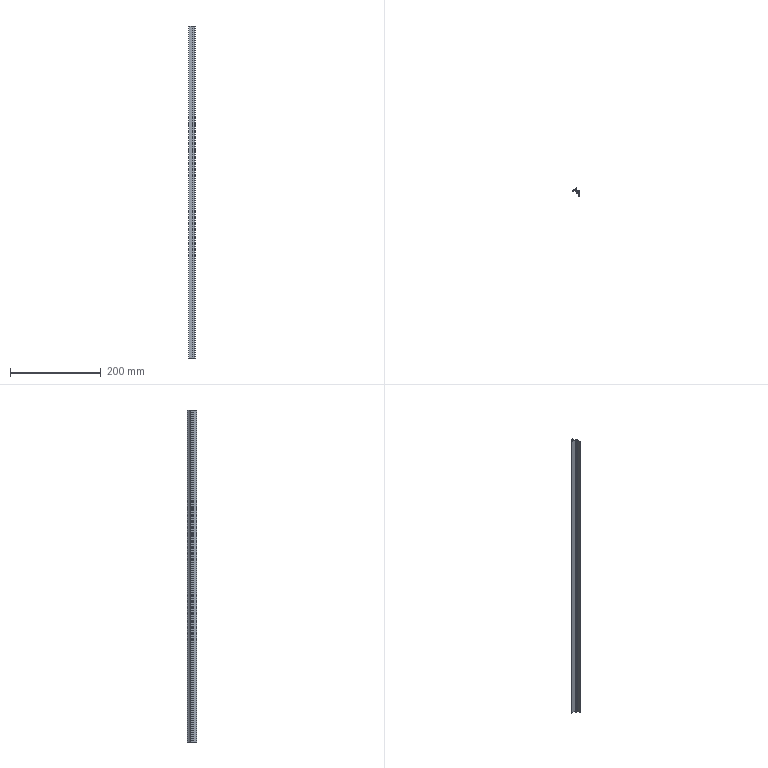Part | SolidWorks | features BaseBody 1, ICE 1, MoveFace 1 | 1 solid | 27 faces | box 14 x 20.3 x 730 mm | volume 37168 mm3 | plane 20 | cylinder 7 | commonest cylinder face diameters 0.387 x2 0.8 x2 0.4 x1 20 x1 22 x1
STEP:
#1=CARTESIAN_POINT('',(-5.304,-0.625,200.));
#2=VERTEX_POINT('',#1);
#3=CARTESIAN_POINT('',(-5.449,-0.8125,200.));
#4=VERTEX_POINT('',#3);
#5=CARTESIAN_POINT('',(-5.255,-0.8125,200.));
#6=DIRECTION('',(0.,0.,1.));
#7=DIRECTION('',(-1.,0.,0.));
#8=AXIS2_PLACEMENT_3D('',#5,#6,#7);
#9=CIRCLE('',#8,0.1937);
#10=EDGE_CURVE('',#2,#4,#9,.T.);
#11=ORIENTED_EDGE('',*,*,#10,.T.);
#12=CARTESIAN_POINT('',(-5.449,-0.8125,-530.));
#13=VERTEX_POINT('',#12);
#14=CARTESIAN_POINT('',(-5.449,-0.8125,230.));
#15=DIRECTION('',(0.,0.,-1.));
#16=VECTOR('',#15,1000.);
#17=LINE('',#14,#16);
#18=EDGE_CURVE('',#4,#13,#17,.T.);
#19=ORIENTED_EDGE('',*,*,#18,.T.);
#20=CARTESIAN_POINT('',(-5.304,-0.625,-530.));
#21=VERTEX_POINT('',#20);
#22=CARTESIAN_POINT('',(-5.255,-0.8125,-530.));
#23=DIRECTION('',(0.,0.,-1.));
#24=DIRECTION('',(1.,0.,0.));
#25=AXIS2_PLACEMENT_3D('',#22,#23,#24);
#26=CIRCLE('',#25,0.1937);
#27=EDGE_CURVE('',#13,#21,#26,.T.);
#28=ORIENTED_EDGE('',*,*,#27,.T.);
#29=CARTESIAN_POINT('',(-5.304,-0.625,230.));
#30=DIRECTION('',(0.,0.,-1.));
#31=VECTOR('',#30,1000.);
#32=LINE('',#29,#31);
#33=EDGE_CURVE('',#2,#21,#32,.T.);
#34=ORIENTED_EDGE('',*,*,#33,.F.);
#35=EDGE_LOOP('',(#11,#19,#28,#34));
#36=FACE_OUTER_BOUND('',#35,.T.);
#37=CARTESIAN_POINT('',(-5.255,-0.8125,230.));
#38=DIRECTION('',(0.,0.,-1.));
#39=DIRECTION('',(-1.,0.,0.));
#40=AXIS2_PLACEMENT_3D('',#37,#38,#39);
#41=CYLINDRICAL_SURFACE('',#40,0.1937);
#42=ADVANCED_FACE('',(#36),#41,.F.);
#43=CARTESIAN_POINT('',(5.,-1.,-530.));
#44=VERTEX_POINT('',#43);
#45=CARTESIAN_POINT('',(5.,-14.3,-530.));
#46=VERTEX_POINT('',#45);
#47=CARTESIAN_POINT('',(5.,29.623,-530.));
#48=DIRECTION('',(0.,-1.,0.));
#49=VECTOR('',#48,1000.);
#50=LINE('',#47,#49);
#51=EDGE_CURVE('',#44,#46,#50,.T.);
#52=ORIENTED_EDGE('',*,*,#51,.F.);
#53=CARTESIAN_POINT('',(5.,-1.,200.));
#54=VERTEX_POINT('',#53);
#55=CARTESIAN_POINT('',(5.,-1.,230.));
#56=DIRECTION('',(0.,0.,-1.));
#57=VECTOR('',#56,1000.);
#58=LINE('',#55,#57);
#59=EDGE_CURVE('',#54,#44,#58,.T.);
#60=ORIENTED_EDGE('',*,*,#59,.F.);
#61=CARTESIAN_POINT('',(5.,-14.3,200.));
#62=VERTEX_POINT('',#61);
#63=CARTESIAN_POINT('',(5.,-14.3,200.));
#64=DIRECTION('',(0.,1.,0.));
#65=VECTOR('',#64,1000.);
#66=LINE('',#63,#65);
#67=EDGE_CURVE('',#62,#54,#66,.T.);
#68=ORIENTED_EDGE('',*,*,#67,.F.);
#69=CARTESIAN_POINT('',(5.,-14.3,230.));
#70=DIRECTION('',(0.,0.,1.));
#71=VECTOR('',#70,1000.);
#72=LINE('',#69,#71);
#73=EDGE_CURVE('',#46,#62,#72,.T.);
#74=ORIENTED_EDGE('',*,*,#73,.F.);
#75=EDGE_LOOP('',(#52,#60,#68,#74));
#76=FACE_OUTER_BOUND('',#75,.T.);
#77=CARTESIAN_POINT('',(5.,-14.3,230.));
#78=DIRECTION('',(-1.,0.,0.));
#79=DIRECTION('',(0.,0.,1.));
#80=AXIS2_PLACEMENT_3D('',#77,#78,#79);
#81=PLANE('',#80);
#82=ADVANCED_FACE('',(#76),#81,.F.);
#83=CARTESIAN_POINT('',(-9.,-2.,-530.));
#84=VERTEX_POINT('',#83);
#85=CARTESIAN_POINT('',(-9.,-2.,200.));
#86=VERTEX_POINT('',#85);
#87=CARTESIAN_POINT('',(-9.,-2.,230.));
#88=DIRECTION('',(0.,0.,1.));
#89=VECTOR('',#88,1000.);
#90=LINE('',#87,#89);
#91=EDGE_CURVE('',#84,#86,#90,.T.);
#92=ORIENTED_EDGE('',*,*,#91,.F.);
#93=CARTESIAN_POINT('',(0.9,-2.,-530.));
#94=VERTEX_POINT('',#93);
#95=CARTESIAN_POINT('',(5.,-2.,-530.));
#96=DIRECTION('',(-1.,0.,0.));
#97=VECTOR('',#96,1000.);
#98=LINE('',#95,#97);
#99=EDGE_CURVE('',#94,#84,#98,.T.);
#100=ORIENTED_EDGE('',*,*,#99,.F.);
#101=CARTESIAN_POINT('',(0.9,-2.,200.));
#102=VERTEX_POINT('',#101);
#103=CARTESIAN_POINT('',(0.9,-2.,230.));
#104=DIRECTION('',(0.,0.,-1.));
#105=VECTOR('',#104,1000.);
#106=LINE('',#103,#105);
#107=EDGE_CURVE('',#102,#94,#106,.T.);
#108=ORIENTED_EDGE('',*,*,#107,.F.);
#109=CARTESIAN_POINT('',(5.,-2.,200.));
#110=DIRECTION('',(1.,0.,0.));
#111=VECTOR('',#110,1000.);
#112=LINE('',#109,#111);
#113=EDGE_CURVE('',#86,#102,#112,.T.);
#114=ORIENTED_EDGE('',*,*,#113,.F.);
#115=EDGE_LOOP('',(#92,#100,#108,#114));
#116=FACE_OUTER_BOUND('',#115,.T.);
#117=CARTESIAN_POINT('',(-9.,-2.,230.));
#118=DIRECTION('',(0.,1.,0.));
#119=DIRECTION('',(0.,0.,1.));
#120=AXIS2_PLACEMENT_3D('',#117,#118,#119);
#121=PLANE('',#120);
#122=ADVANCED_FACE('',(#116),#121,.F.);
#123=CARTESIAN_POINT('',(4.,-6.,200.));
#124=VERTEX_POINT('',#123);
#125=CARTESIAN_POINT('',(4.,-3.,200.));
#126=VERTEX_POINT('',#125);
#127=CARTESIAN_POINT('',(4.,29.623,200.));
#128=DIRECTION('',(0.,1.,0.));
#129=VECTOR('',#128,1000.);
#130=LINE('',#127,#129);
#131=EDGE_CURVE('',#124,#126,#130,.T.);
#132=ORIENTED_EDGE('',*,*,#131,.F.);
#133=CARTESIAN_POINT('',(1.,-6.,200.));
#134=VERTEX_POINT('',#133);
#135=CARTESIAN_POINT('',(5.,-6.,200.));
#136=DIRECTION('',(1.,0.,0.));
#137=VECTOR('',#136,1000.);
#138=LINE('',#135,#137);
#139=EDGE_CURVE('',#134,#124,#138,.T.);
#140=ORIENTED_EDGE('',*,*,#139,.F.);
#141=CARTESIAN_POINT('',(1.,-6.7,200.));
#142=VERTEX_POINT('',#141);
#143=CARTESIAN_POINT('',(1.,-6.,200.));
#144=DIRECTION('',(0.,-1.,0.));
#145=VECTOR('',#144,1000.);
#146=LINE('',#143,#145);
#147=EDGE_CURVE('',#134,#142,#146,.T.);
#148=ORIENTED_EDGE('',*,*,#147,.T.);
#149=CARTESIAN_POINT('',(-1.7,-6.7,200.));
#150=VERTEX_POINT('',#149);
#151=CARTESIAN_POINT('',(5.,-6.7,200.));
#152=DIRECTION('',(1.,0.,0.));
#153=VECTOR('',#152,1000.);
#154=LINE('',#151,#153);
#155=EDGE_CURVE('',#150,#142,#154,.T.);
#156=ORIENTED_EDGE('',*,*,#155,.F.);
#157=CARTESIAN_POINT('',(-1.7,-7.7,200.));
#158=VERTEX_POINT('',#157);
#159=CARTESIAN_POINT('',(-1.7,-6.7,200.));
#160=DIRECTION('',(0.,-1.,0.));
#161=VECTOR('',#160,1000.);
#162=LINE('',#159,#161);
#163=EDGE_CURVE('',#150,#158,#162,.T.);
#164=ORIENTED_EDGE('',*,*,#163,.T.);
#165=CARTESIAN_POINT('',(4.,-7.7,200.));
#166=VERTEX_POINT('',#165);
#167=CARTESIAN_POINT('',(5.,-7.7,200.));
#168=DIRECTION('',(-1.,0.,0.));
#169=VECTOR('',#168,1000.);
#170=LINE('',#167,#169);
#171=EDGE_CURVE('',#166,#158,#170,.T.);
#172=ORIENTED_EDGE('',*,*,#171,.F.);
#173=CARTESIAN_POINT('',(4.,-14.3,200.));
#174=VERTEX_POINT('',#173);
#175=CARTESIAN_POINT('',(4.,29.623,200.));
#176=DIRECTION('',(0.,1.,0.));
#177=VECTOR('',#176,1000.);
#178=LINE('',#175,#177);
#179=EDGE_CURVE('',#174,#166,#178,.T.);
#180=ORIENTED_EDGE('',*,*,#179,.F.);
#181=CARTESIAN_POINT('',(5.,-14.3,200.));
#182=DIRECTION('',(-1.,0.,0.));
#183=VECTOR('',#182,1000.);
#184=LINE('',#181,#183);
#185=EDGE_CURVE('',#62,#174,#184,.T.);
#186=ORIENTED_EDGE('',*,*,#185,.F.);
#187=ORIENTED_EDGE('',*,*,#67,.T.);
#188=CARTESIAN_POINT('',(-5.207,-1.,200.));
#189=VERTEX_POINT('',#188);
#190=CARTESIAN_POINT('',(5.,-1.,200.));
#191=DIRECTION('',(1.,0.,0.));
#192=VECTOR('',#191,1000.);
#193=LINE('',#190,#192);
#194=EDGE_CURVE('',#189,#54,#193,.T.);
#195=ORIENTED_EDGE('',*,*,#194,.F.);
#196=CARTESIAN_POINT('',(-5.255,-0.8125,200.));
#197=DIRECTION('',(0.,0.,1.));
#198=DIRECTION('',(-1.,0.,0.));
#199=AXIS2_PLACEMENT_3D('',#196,#197,#198);
#200=CIRCLE('',#199,0.1937);
#201=EDGE_CURVE('',#4,#189,#200,.T.);
#202=ORIENTED_EDGE('',*,*,#201,.F.);
#203=ORIENTED_EDGE('',*,*,#10,.F.);
#204=CARTESIAN_POINT('',(-1.368,3.063,200.));
#205=VERTEX_POINT('',#204);
#206=CARTESIAN_POINT('',(-10.628,9.,200.));
#207=DIRECTION('',(0.,0.,1.));
#208=DIRECTION('',(-1.,0.,0.));
#209=AXIS2_PLACEMENT_3D('',#206,#207,#208);
#210=CIRCLE('',#209,11.);
#211=EDGE_CURVE('',#2,#205,#210,.T.);
#212=ORIENTED_EDGE('',*,*,#211,.T.);
#213=CARTESIAN_POINT('',(-1.,2.955,200.));
#214=VERTEX_POINT('',#213);
#215=CARTESIAN_POINT('',(-1.2,2.955,200.));
#216=DIRECTION('',(0.,0.,1.));
#217=DIRECTION('',(-1.,0.,0.));
#218=AXIS2_PLACEMENT_3D('',#215,#216,#217);
#219=CIRCLE('',#218,0.2);
#220=EDGE_CURVE('',#214,#205,#219,.T.);
#221=ORIENTED_EDGE('',*,*,#220,.F.);
#222=CARTESIAN_POINT('',(-1.,1.5,200.));
#223=VERTEX_POINT('',#222);
#224=CARTESIAN_POINT('',(-1.,2.955,200.));
#225=DIRECTION('',(0.,1.,0.));
#226=VECTOR('',#225,1000.);
#227=LINE('',#224,#226);
#228=EDGE_CURVE('',#223,#214,#227,.T.);
#229=ORIENTED_EDGE('',*,*,#228,.F.);
#230=CARTESIAN_POINT('',(0.,1.5,200.));
#231=VERTEX_POINT('',#230);
#232=CARTESIAN_POINT('',(-1.,1.5,200.));
#233=DIRECTION('',(-1.,0.,0.));
#234=VECTOR('',#233,1000.);
#235=LINE('',#232,#234);
#236=EDGE_CURVE('',#231,#223,#235,.T.);
#237=ORIENTED_EDGE('',*,*,#236,.F.);
#238=CARTESIAN_POINT('',(0.,6.,200.));
#239=VERTEX_POINT('',#238);
#240=CARTESIAN_POINT('',(0.,1.5,200.));
#241=DIRECTION('',(0.,-1.,0.));
#242=VECTOR('',#241,1000.);
#243=LINE('',#240,#242);
#244=EDGE_CURVE('',#239,#231,#243,.T.);
#245=ORIENTED_EDGE('',*,*,#244,.F.);
#246=CARTESIAN_POINT('',(-0.8,6.,200.));
#247=VERTEX_POINT('',#246);
#248=CARTESIAN_POINT('',(0.,6.,200.));
#249=DIRECTION('',(1.,0.,0.));
#250=VECTOR('',#249,1000.);
#251=LINE('',#248,#250);
#252=EDGE_CURVE('',#247,#239,#251,.T.);
#253=ORIENTED_EDGE('',*,*,#252,.F.);
#254=CARTESIAN_POINT('',(-1.178,5.731,200.));
#255=VERTEX_POINT('',#254);
#256=CARTESIAN_POINT('',(-0.8,5.6,200.));
#257=DIRECTION('',(0.,0.,1.));
#258=DIRECTION('',(-1.,0.,0.));
#259=AXIS2_PLACEMENT_3D('',#256,#257,#258);
#260=CIRCLE('',#259,0.4);
#261=EDGE_CURVE('',#247,#255,#260,.T.);
#262=ORIENTED_EDGE('',*,*,#261,.T.);
#263=CARTESIAN_POINT('',(-8.678,-0.8077,200.));
#264=VERTEX_POINT('',#263);
#265=CARTESIAN_POINT('',(-10.628,9.,200.));
#266=DIRECTION('',(0.,0.,1.));
#267=DIRECTION('',(-1.,0.,0.));
#268=AXIS2_PLACEMENT_3D('',#265,#266,#267);
#269=CIRCLE('',#268,10.);
#270=EDGE_CURVE('',#264,#255,#269,.T.);
#271=ORIENTED_EDGE('',*,*,#270,.F.);
#272=CARTESIAN_POINT('',(-9.,-1.2,200.));
#273=VERTEX_POINT('',#272);
#274=CARTESIAN_POINT('',(-8.6,-1.2,200.));
#275=DIRECTION('',(0.,0.,1.));
#276=DIRECTION('',(-1.,0.,0.));
#277=AXIS2_PLACEMENT_3D('',#274,#275,#276);
#278=CIRCLE('',#277,0.4);
#279=EDGE_CURVE('',#264,#273,#278,.T.);
#280=ORIENTED_EDGE('',*,*,#279,.T.);
#281=CARTESIAN_POINT('',(-9.,8.,200.));
#282=DIRECTION('',(0.,-1.,0.));
#283=VECTOR('',#282,1000.);
#284=LINE('',#281,#283);
#285=EDGE_CURVE('',#273,#86,#284,.T.);
#286=ORIENTED_EDGE('',*,*,#285,.T.);
#287=ORIENTED_EDGE('',*,*,#113,.T.);
#288=CARTESIAN_POINT('',(0.9,-3.,200.));
#289=VERTEX_POINT('',#288);
#290=CARTESIAN_POINT('',(0.9,29.623,200.));
#291=DIRECTION('',(0.,1.,0.));
#292=VECTOR('',#291,1000.);
#293=LINE('',#290,#292);
#294=EDGE_CURVE('',#289,#102,#293,.T.);
#295=ORIENTED_EDGE('',*,*,#294,.F.);
#296=CARTESIAN_POINT('',(5.,-3.,200.));
#297=DIRECTION('',(-1.,0.,0.));
#298=VECTOR('',#297,1000.);
#299=LINE('',#296,#298);
#300=EDGE_CURVE('',#126,#289,#299,.T.);
#301=ORIENTED_EDGE('',*,*,#300,.F.);
#302=EDGE_LOOP('',(#132,#140,#148,#156,#164,#172,#180,#186,#187,#195,#202,#203,#212,#221,#229,#237,#245,#253,#262,#271,#280,#286,#287,#295,#301));
#303=FACE_OUTER_BOUND('',#302,.T.);
#304=CARTESIAN_POINT('',(5.,29.623,200.));
#305=DIRECTION('',(0.,0.,-1.));
#306=DIRECTION('',(-1.,0.,0.));
#307=AXIS2_PLACEMENT_3D('',#304,#305,#306);
#308=PLANE('',#307);
#309=ADVANCED_FACE('',(#303),#308,.F.);
#310=ORIENTED_EDGE('',*,*,#185,.T.);
#311=CARTESIAN_POINT('',(4.,-14.3,-530.));
#312=VERTEX_POINT('',#311);
#313=CARTESIAN_POINT('',(4.,-14.3,230.));
#314=DIRECTION('',(0.,0.,1.));
#315=VECTOR('',#314,1000.);
#316=LINE('',#313,#315);
#317=EDGE_CURVE('',#312,#174,#316,.T.);
#318=ORIENTED_EDGE('',*,*,#317,.F.);
#319=CARTESIAN_POINT('',(5.,-14.3,-530.));
#320=DIRECTION('',(-1.,0.,0.));
#321=VECTOR('',#320,1000.);
#322=LINE('',#319,#321);
#323=EDGE_CURVE('',#46,#312,#322,.T.);
#324=ORIENTED_EDGE('',*,*,#323,.F.);
#325=ORIENTED_EDGE('',*,*,#73,.T.);
#326=EDGE_LOOP('',(#310,#318,#324,#325));
#327=FACE_OUTER_BOUND('',#326,.T.);
#328=CARTESIAN_POINT('',(4.,-14.3,230.));
#329=DIRECTION('',(0.,1.,0.));
#330=DIRECTION('',(0.,0.,1.));
#331=AXIS2_PLACEMENT_3D('',#328,#329,#330);
#332=PLANE('',#331);
#333=ADVANCED_FACE('',(#327),#332,.F.);
#334=ORIENTED_EDGE('',*,*,#51,.T.);
#335=ORIENTED_EDGE('',*,*,#323,.T.);
#336=CARTESIAN_POINT('',(4.,-7.7,-530.));
#337=VERTEX_POINT('',#336);
#338=CARTESIAN_POINT('',(4.,-7.7,-530.));
#339=DIRECTION('',(0.,-1.,0.));
#340=VECTOR('',#339,1000.);
#341=LINE('',#338,#340);
#342=EDGE_CURVE('',#337,#312,#341,.T.);
#343=ORIENTED_EDGE('',*,*,#342,.F.);
#344=CARTESIAN_POINT('',(-1.7,-7.7,-530.));
#345=VERTEX_POINT('',#344);
#346=CARTESIAN_POINT('',(-1.7,-7.7,-530.));
#347=DIRECTION('',(1.,0.,0.));
#348=VECTOR('',#347,1000.);
#349=LINE('',#346,#348);
#350=EDGE_CURVE('',#345,#337,#349,.T.);
#351=ORIENTED_EDGE('',*,*,#350,.F.);
#352=CARTESIAN_POINT('',(-1.7,-6.7,-530.));
#353=VERTEX_POINT('',#352);
#354=CARTESIAN_POINT('',(-1.7,29.623,-530.));
#355=DIRECTION('',(0.,1.,0.));
#356=VECTOR('',#355,1000.);
#357=LINE('',#354,#356);
#358=EDGE_CURVE('',#345,#353,#357,.T.);
#359=ORIENTED_EDGE('',*,*,#358,.T.);
#360=CARTESIAN_POINT('',(1.,-6.7,-530.));
#361=VERTEX_POINT('',#360);
#362=CARTESIAN_POINT('',(1.,-6.7,-530.));
#363=DIRECTION('',(-1.,0.,0.));
#364=VECTOR('',#363,1000.);
#365=LINE('',#362,#364);
#366=EDGE_CURVE('',#361,#353,#365,.T.);
#367=ORIENTED_EDGE('',*,*,#366,.F.);
#368=CARTESIAN_POINT('',(1.,-6.,-530.));
#369=VERTEX_POINT('',#368);
#370=CARTESIAN_POINT('',(1.,29.623,-530.));
#371=DIRECTION('',(0.,1.,0.));
#372=VECTOR('',#371,1000.);
#373=LINE('',#370,#372);
#374=EDGE_CURVE('',#361,#369,#373,.T.);
#375=ORIENTED_EDGE('',*,*,#374,.T.);
#376=CARTESIAN_POINT('',(4.,-6.,-530.));
#377=VERTEX_POINT('',#376);
#378=CARTESIAN_POINT('',(4.,-6.,-530.));
#379=DIRECTION('',(-1.,0.,0.));
#380=VECTOR('',#379,1000.);
#381=LINE('',#378,#380);
#382=EDGE_CURVE('',#377,#369,#381,.T.);
#383=ORIENTED_EDGE('',*,*,#382,.F.);
#384=CARTESIAN_POINT('',(4.,-3.,-530.));
#385=VERTEX_POINT('',#384);
#386=CARTESIAN_POINT('',(4.,-3.,-530.));
#387=DIRECTION('',(0.,-1.,0.));
#388=VECTOR('',#387,1000.);
#389=LINE('',#386,#388);
#390=EDGE_CURVE('',#385,#377,#389,.T.);
#391=ORIENTED_EDGE('',*,*,#390,.F.);
#392=CARTESIAN_POINT('',(0.9,-3.,-530.));
#393=VERTEX_POINT('',#392);
#394=CARTESIAN_POINT('',(0.9,-3.,-530.));
#395=DIRECTION('',(1.,0.,0.));
#396=VECTOR('',#395,1000.);
#397=LINE('',#394,#396);
#398=EDGE_CURVE('',#393,#385,#397,.T.);
#399=ORIENTED_EDGE('',*,*,#398,.F.);
#400=CARTESIAN_POINT('',(0.9,-2.,-530.));
#401=DIRECTION('',(0.,-1.,0.));
#402=VECTOR('',#401,1000.);
#403=LINE('',#400,#402);
#404=EDGE_CURVE('',#94,#393,#403,.T.);
#405=ORIENTED_EDGE('',*,*,#404,.F.);
#406=ORIENTED_EDGE('',*,*,#99,.T.);
#407=CARTESIAN_POINT('',(-9.,-1.2,-530.));
#408=VERTEX_POINT('',#407);
#409=CARTESIAN_POINT('',(-9.,-1.2,-530.));
#410=DIRECTION('',(0.,-1.,0.));
#411=VECTOR('',#410,1000.);
#412=LINE('',#409,#411);
#413=EDGE_CURVE('',#408,#84,#412,.T.);
#414=ORIENTED_EDGE('',*,*,#413,.F.);
#415=CARTESIAN_POINT('',(-8.678,-0.8077,-530.));
#416=VERTEX_POINT('',#415);
#417=CARTESIAN_POINT('',(-8.6,-1.2,-530.));
#418=DIRECTION('',(0.,0.,-1.));
#419=DIRECTION('',(1.,0.,0.));
#420=AXIS2_PLACEMENT_3D('',#417,#418,#419);
#421=CIRCLE('',#420,0.4);
#422=EDGE_CURVE('',#408,#416,#421,.T.);
#423=ORIENTED_EDGE('',*,*,#422,.T.);
#424=CARTESIAN_POINT('',(-1.178,5.731,-530.));
#425=VERTEX_POINT('',#424);
#426=CARTESIAN_POINT('',(-10.628,9.,-530.));
#427=DIRECTION('',(0.,0.,-1.));
#428=DIRECTION('',(1.,0.,0.));
#429=AXIS2_PLACEMENT_3D('',#426,#427,#428);
#430=CIRCLE('',#429,10.);
#431=EDGE_CURVE('',#425,#416,#430,.T.);
#432=ORIENTED_EDGE('',*,*,#431,.F.);
#433=CARTESIAN_POINT('',(-0.8,6.,-530.));
#434=VERTEX_POINT('',#433);
#435=CARTESIAN_POINT('',(-0.8,5.6,-530.));
#436=DIRECTION('',(0.,0.,-1.));
#437=DIRECTION('',(1.,0.,0.));
#438=AXIS2_PLACEMENT_3D('',#435,#436,#437);
#439=CIRCLE('',#438,0.4);
#440=EDGE_CURVE('',#425,#434,#439,.T.);
#441=ORIENTED_EDGE('',*,*,#440,.T.);
#442=CARTESIAN_POINT('',(0.,6.,-530.));
#443=VERTEX_POINT('',#442);
#444=CARTESIAN_POINT('',(0.,6.,-530.));
#445=DIRECTION('',(-1.,0.,0.));
#446=VECTOR('',#445,1000.);
#447=LINE('',#444,#446);
#448=EDGE_CURVE('',#443,#434,#447,.T.);
#449=ORIENTED_EDGE('',*,*,#448,.F.);
#450=CARTESIAN_POINT('',(0.,1.5,-530.));
#451=VERTEX_POINT('',#450);
#452=CARTESIAN_POINT('',(0.,1.5,-530.));
#453=DIRECTION('',(0.,1.,0.));
#454=VECTOR('',#453,1000.);
#455=LINE('',#452,#454);
#456=EDGE_CURVE('',#451,#443,#455,.T.);
#457=ORIENTED_EDGE('',*,*,#456,.F.);
#458=CARTESIAN_POINT('',(-1.,1.5,-530.));
#459=VERTEX_POINT('',#458);
#460=CARTESIAN_POINT('',(-1.,1.5,-530.));
#461=DIRECTION('',(1.,0.,0.));
#462=VECTOR('',#461,1000.);
#463=LINE('',#460,#462);
#464=EDGE_CURVE('',#459,#451,#463,.T.);
#465=ORIENTED_EDGE('',*,*,#464,.F.);
#466=CARTESIAN_POINT('',(-1.,2.955,-530.));
#467=VERTEX_POINT('',#466);
#468=CARTESIAN_POINT('',(-1.,2.955,-530.));
#469=DIRECTION('',(0.,-1.,0.));
#470=VECTOR('',#469,1000.);
#471=LINE('',#468,#470);
#472=EDGE_CURVE('',#467,#459,#471,.T.);
#473=ORIENTED_EDGE('',*,*,#472,.F.);
#474=CARTESIAN_POINT('',(-1.368,3.063,-530.));
#475=VERTEX_POINT('',#474);
#476=CARTESIAN_POINT('',(-1.2,2.955,-530.));
#477=DIRECTION('',(0.,0.,-1.));
#478=DIRECTION('',(1.,0.,0.));
#479=AXIS2_PLACEMENT_3D('',#476,#477,#478);
#480=CIRCLE('',#479,0.2);
#481=EDGE_CURVE('',#475,#467,#480,.T.);
#482=ORIENTED_EDGE('',*,*,#481,.F.);
#483=CARTESIAN_POINT('',(-10.628,9.,-530.));
#484=DIRECTION('',(0.,0.,-1.));
#485=DIRECTION('',(1.,0.,0.));
#486=AXIS2_PLACEMENT_3D('',#483,#484,#485);
#487=CIRCLE('',#486,11.);
#488=EDGE_CURVE('',#475,#21,#487,.T.);
#489=ORIENTED_EDGE('',*,*,#488,.T.);
#490=ORIENTED_EDGE('',*,*,#27,.F.);
#491=CARTESIAN_POINT('',(-5.207,-1.,-530.));
#492=VERTEX_POINT('',#491);
#493=CARTESIAN_POINT('',(-5.255,-0.8125,-530.));
#494=DIRECTION('',(0.,0.,-1.));
#495=DIRECTION('',(1.,0.,0.));
#496=AXIS2_PLACEMENT_3D('',#493,#494,#495);
#497=CIRCLE('',#496,0.1937);
#498=EDGE_CURVE('',#492,#13,#497,.T.);
#499=ORIENTED_EDGE('',*,*,#498,.F.);
#500=CARTESIAN_POINT('',(5.,-1.,-530.));
#501=DIRECTION('',(-1.,0.,0.));
#502=VECTOR('',#501,1000.);
#503=LINE('',#500,#502);
#504=EDGE_CURVE('',#44,#492,#503,.T.);
#505=ORIENTED_EDGE('',*,*,#504,.F.);
#506=EDGE_LOOP('',(#334,#335,#343,#351,#359,#367,#375,#383,#391,#399,#405,#406,#414,#423,#432,#441,#449,#457,#465,#473,#482,#489,#490,#499,#505));
#507=FACE_OUTER_BOUND('',#506,.T.);
#508=CARTESIAN_POINT('',(5.,29.623,-530.));
#509=DIRECTION('',(0.,0.,1.));
#510=DIRECTION('',(1.,0.,0.));
#511=AXIS2_PLACEMENT_3D('',#508,#509,#510);
#512=PLANE('',#511);
#513=ADVANCED_FACE('',(#507),#512,.F.);
#514=ORIENTED_EDGE('',*,*,#59,.T.);
#515=ORIENTED_EDGE('',*,*,#504,.T.);
#516=CARTESIAN_POINT('',(-5.207,-1.,230.));
#517=DIRECTION('',(0.,0.,-1.));
#518=VECTOR('',#517,1000.);
#519=LINE('',#516,#518);
#520=EDGE_CURVE('',#189,#492,#519,.T.);
#521=ORIENTED_EDGE('',*,*,#520,.F.);
#522=ORIENTED_EDGE('',*,*,#194,.T.);
#523=EDGE_LOOP('',(#514,#515,#521,#522));
#524=FACE_OUTER_BOUND('',#523,.T.);
#525=CARTESIAN_POINT('',(5.,-1.,230.));
#526=DIRECTION('',(0.,-1.,0.));
#527=DIRECTION('',(0.,0.,-1.));
#528=AXIS2_PLACEMENT_3D('',#525,#526,#527);
#529=PLANE('',#528);
#530=ADVANCED_FACE('',(#524),#529,.F.);
#531=CARTESIAN_POINT('',(-9.,-1.2,230.));
#532=DIRECTION('',(0.,0.,1.));
#533=VECTOR('',#532,1000.);
#534=LINE('',#531,#533);
#535=EDGE_CURVE('',#408,#273,#534,.T.);
#536=ORIENTED_EDGE('',*,*,#535,.F.);
#537=ORIENTED_EDGE('',*,*,#413,.T.);
#538=ORIENTED_EDGE('',*,*,#91,.T.);
#539=ORIENTED_EDGE('',*,*,#285,.F.);
#540=EDGE_LOOP('',(#536,#537,#538,#539));
#541=FACE_OUTER_BOUND('',#540,.T.);
#542=CARTESIAN_POINT('',(-9.,-1.2,230.));
#543=DIRECTION('',(1.,0.,0.));
#544=DIRECTION('',(0.,0.,-1.));
#545=AXIS2_PLACEMENT_3D('',#542,#543,#544);
#546=PLANE('',#545);
#547=ADVANCED_FACE('',(#541),#546,.F.);
#548=ORIENTED_EDGE('',*,*,#294,.T.);
#549=ORIENTED_EDGE('',*,*,#107,.T.);
#550=ORIENTED_EDGE('',*,*,#404,.T.);
#551=CARTESIAN_POINT('',(0.9,-3.,230.));
#552=DIRECTION('',(0.,0.,-1.));
#553=VECTOR('',#552,1000.);
#554=LINE('',#551,#553);
#555=EDGE_CURVE('',#289,#393,#554,.T.);
#556=ORIENTED_EDGE('',*,*,#555,.F.);
#557=EDGE_LOOP('',(#548,#549,#550,#556));
#558=FACE_OUTER_BOUND('',#557,.T.);
#559=CARTESIAN_POINT('',(0.9,-2.,230.));
#560=DIRECTION('',(1.,0.,0.));
#561=DIRECTION('',(0.,0.,-1.));
#562=AXIS2_PLACEMENT_3D('',#559,#560,#561);
#563=PLANE('',#562);
#564=ADVANCED_FACE('',(#558),#563,.F.);
#565=ORIENTED_EDGE('',*,*,#300,.T.);
#566=ORIENTED_EDGE('',*,*,#555,.T.);
#567=ORIENTED_EDGE('',*,*,#398,.T.);
#568=CARTESIAN_POINT('',(4.,-3.,230.));
#569=DIRECTION('',(0.,0.,-1.));
#570=VECTOR('',#569,1000.);
#571=LINE('',#568,#570);
#572=EDGE_CURVE('',#126,#385,#571,.T.);
#573=ORIENTED_EDGE('',*,*,#572,.F.);
#574=EDGE_LOOP('',(#565,#566,#567,#573));
#575=FACE_OUTER_BOUND('',#574,.T.);
#576=CARTESIAN_POINT('',(0.9,-3.,230.));
#577=DIRECTION('',(0.,1.,0.));
#578=DIRECTION('',(0.,0.,1.));
#579=AXIS2_PLACEMENT_3D('',#576,#577,#578);
#580=PLANE('',#579);
#581=ADVANCED_FACE('',(#575),#580,.F.);
#582=ORIENTED_EDGE('',*,*,#131,.T.);
#583=ORIENTED_EDGE('',*,*,#572,.T.);
#584=ORIENTED_EDGE('',*,*,#390,.T.);
#585=CARTESIAN_POINT('',(4.,-6.,230.));
#586=DIRECTION('',(0.,0.,-1.));
#587=VECTOR('',#586,1000.);
#588=LINE('',#585,#587);
#589=EDGE_CURVE('',#124,#377,#588,.T.);
#590=ORIENTED_EDGE('',*,*,#589,.F.);
#591=EDGE_LOOP('',(#582,#583,#584,#590));
#592=FACE_OUTER_BOUND('',#591,.T.);
#593=CARTESIAN_POINT('',(4.,-3.,230.));
#594=DIRECTION('',(1.,0.,0.));
#595=DIRECTION('',(0.,0.,-1.));
#596=AXIS2_PLACEMENT_3D('',#593,#594,#595);
#597=PLANE('',#596);
#598=ADVANCED_FACE('',(#592),#597,.F.);
#599=ORIENTED_EDGE('',*,*,#139,.T.);
#600=ORIENTED_EDGE('',*,*,#589,.T.);
#601=ORIENTED_EDGE('',*,*,#382,.T.);
#602=CARTESIAN_POINT('',(1.,-6.,230.));
#603=DIRECTION('',(0.,0.,-1.));
#604=VECTOR('',#603,1000.);
#605=LINE('',#602,#604);
#606=EDGE_CURVE('',#134,#369,#605,.T.);
#607=ORIENTED_EDGE('',*,*,#606,.F.);
#608=EDGE_LOOP('',(#599,#600,#601,#607));
#609=FACE_OUTER_BOUND('',#608,.T.);
#610=CARTESIAN_POINT('',(4.,-6.,230.));
#611=DIRECTION('',(0.,-1.,0.));
#612=DIRECTION('',(0.,0.,-1.));
#613=AXIS2_PLACEMENT_3D('',#610,#611,#612);
#614=PLANE('',#613);
#615=ADVANCED_FACE('',(#609),#614,.F.);
#616=ORIENTED_EDGE('',*,*,#155,.T.);
#617=CARTESIAN_POINT('',(1.,-6.7,230.));
#618=DIRECTION('',(0.,0.,1.));
#619=VECTOR('',#618,1000.);
#620=LINE('',#617,#619);
#621=EDGE_CURVE('',#361,#142,#620,.T.);
#622=ORIENTED_EDGE('',*,*,#621,.F.);
#623=ORIENTED_EDGE('',*,*,#366,.T.);
#624=CARTESIAN_POINT('',(-1.7,-6.7,230.));
#625=DIRECTION('',(0.,0.,-1.));
#626=VECTOR('',#625,1000.);
#627=LINE('',#624,#626);
#628=EDGE_CURVE('',#150,#353,#627,.T.);
#629=ORIENTED_EDGE('',*,*,#628,.F.);
#630=EDGE_LOOP('',(#616,#622,#623,#629));
#631=FACE_OUTER_BOUND('',#630,.T.);
#632=CARTESIAN_POINT('',(1.,-6.7,230.));
#633=DIRECTION('',(0.,-1.,0.));
#634=DIRECTION('',(0.,0.,-1.));
#635=AXIS2_PLACEMENT_3D('',#632,#633,#634);
#636=PLANE('',#635);
#637=ADVANCED_FACE('',(#631),#636,.F.);
#638=ORIENTED_EDGE('',*,*,#171,.T.);
#639=CARTESIAN_POINT('',(-1.7,-7.7,230.));
#640=DIRECTION('',(0.,0.,1.));
#641=VECTOR('',#640,1000.);
#642=LINE('',#639,#641);
#643=EDGE_CURVE('',#345,#158,#642,.T.);
#644=ORIENTED_EDGE('',*,*,#643,.F.);
#645=ORIENTED_EDGE('',*,*,#350,.T.);
#646=CARTESIAN_POINT('',(4.,-7.7,230.));
#647=DIRECTION('',(0.,0.,-1.));
#648=VECTOR('',#647,1000.);
#649=LINE('',#646,#648);
#650=EDGE_CURVE('',#166,#337,#649,.T.);
#651=ORIENTED_EDGE('',*,*,#650,.F.);
#652=EDGE_LOOP('',(#638,#644,#645,#651));
#653=FACE_OUTER_BOUND('',#652,.T.);
#654=CARTESIAN_POINT('',(-1.7,-7.7,230.));
#655=DIRECTION('',(0.,1.,0.));
#656=DIRECTION('',(0.,0.,1.));
#657=AXIS2_PLACEMENT_3D('',#654,#655,#656);
#658=PLANE('',#657);
#659=ADVANCED_FACE('',(#653),#658,.F.);
#660=ORIENTED_EDGE('',*,*,#179,.T.);
#661=ORIENTED_EDGE('',*,*,#650,.T.);
#662=ORIENTED_EDGE('',*,*,#342,.T.);
#663=ORIENTED_EDGE('',*,*,#317,.T.);
#664=EDGE_LOOP('',(#660,#661,#662,#663));
#665=FACE_OUTER_BOUND('',#664,.T.);
#666=CARTESIAN_POINT('',(4.,-7.7,230.));
#667=DIRECTION('',(1.,0.,0.));
#668=DIRECTION('',(0.,0.,-1.));
#669=AXIS2_PLACEMENT_3D('',#666,#667,#668);
#670=PLANE('',#669);
#671=ADVANCED_FACE('',(#665),#670,.F.);
#672=ORIENTED_EDGE('',*,*,#18,.F.);
#673=ORIENTED_EDGE('',*,*,#201,.T.);
#674=ORIENTED_EDGE('',*,*,#520,.T.);
#675=ORIENTED_EDGE('',*,*,#498,.T.);
#676=EDGE_LOOP('',(#672,#673,#674,#675));
#677=FACE_OUTER_BOUND('',#676,.T.);
#678=CARTESIAN_POINT('',(-5.255,-0.8125,230.));
#679=DIRECTION('',(0.,0.,-1.));
#680=DIRECTION('',(-1.,0.,0.));
#681=AXIS2_PLACEMENT_3D('',#678,#679,#680);
#682=CYLINDRICAL_SURFACE('',#681,0.1937);
#683=ADVANCED_FACE('',(#677),#682,.F.);
#684=CARTESIAN_POINT('',(-1.,2.955,230.));
#685=DIRECTION('',(0.,0.,1.));
#686=VECTOR('',#685,1000.);
#687=LINE('',#684,#686);
#688=EDGE_CURVE('',#467,#214,#687,.T.);
#689=ORIENTED_EDGE('',*,*,#688,.F.);
#690=ORIENTED_EDGE('',*,*,#472,.T.);
#691=CARTESIAN_POINT('',(-1.,1.5,230.));
#692=DIRECTION('',(0.,0.,-1.));
#693=VECTOR('',#692,1000.);
#694=LINE('',#691,#693);
#695=EDGE_CURVE('',#223,#459,#694,.T.);
#696=ORIENTED_EDGE('',*,*,#695,.F.);
#697=ORIENTED_EDGE('',*,*,#228,.T.);
#698=EDGE_LOOP('',(#689,#690,#696,#697));
#699=FACE_OUTER_BOUND('',#698,.T.);
#700=CARTESIAN_POINT('',(-1.,2.955,230.));
#701=DIRECTION('',(1.,0.,0.));
#702=DIRECTION('',(0.,0.,-1.));
#703=AXIS2_PLACEMENT_3D('',#700,#701,#702);
#704=PLANE('',#703);
#705=ADVANCED_FACE('',(#699),#704,.F.);
#706=ORIENTED_EDGE('',*,*,#488,.F.);
#707=CARTESIAN_POINT('',(-1.368,3.063,230.));
#708=DIRECTION('',(0.,0.,1.));
#709=VECTOR('',#708,1000.);
#710=LINE('',#707,#709);
#711=EDGE_CURVE('',#475,#205,#710,.T.);
#712=ORIENTED_EDGE('',*,*,#711,.T.);
#713=ORIENTED_EDGE('',*,*,#211,.F.);
#714=ORIENTED_EDGE('',*,*,#33,.T.);
#715=EDGE_LOOP('',(#706,#712,#713,#714));
#716=FACE_OUTER_BOUND('',#715,.T.);
#717=CARTESIAN_POINT('',(-10.628,9.,230.));
#718=DIRECTION('',(0.,0.,-1.));
#719=DIRECTION('',(-1.,0.,0.));
#720=AXIS2_PLACEMENT_3D('',#717,#718,#719);
#721=CYLINDRICAL_SURFACE('',#720,11.);
#722=ADVANCED_FACE('',(#716),#721,.T.);
#723=CARTESIAN_POINT('',(-1.178,5.731,230.));
#724=DIRECTION('',(0.,0.,1.));
#725=VECTOR('',#724,1000.);
#726=LINE('',#723,#725);
#727=EDGE_CURVE('',#425,#255,#726,.T.);
#728=ORIENTED_EDGE('',*,*,#727,.F.);
#729=ORIENTED_EDGE('',*,*,#431,.T.);
#730=CARTESIAN_POINT('',(-8.678,-0.8077,230.));
#731=DIRECTION('',(0.,0.,-1.));
#732=VECTOR('',#731,1000.);
#733=LINE('',#730,#732);
#734=EDGE_CURVE('',#264,#416,#733,.T.);
#735=ORIENTED_EDGE('',*,*,#734,.F.);
#736=ORIENTED_EDGE('',*,*,#270,.T.);
#737=EDGE_LOOP('',(#728,#729,#735,#736));
#738=FACE_OUTER_BOUND('',#737,.T.);
#739=CARTESIAN_POINT('',(-10.628,9.,230.));
#740=DIRECTION('',(0.,0.,-1.));
#741=DIRECTION('',(-1.,0.,0.));
#742=AXIS2_PLACEMENT_3D('',#739,#740,#741);
#743=CYLINDRICAL_SURFACE('',#742,10.);
#744=ADVANCED_FACE('',(#738),#743,.F.);
#745=CARTESIAN_POINT('',(0.,1.5,230.));
#746=DIRECTION('',(0.,0.,1.));
#747=VECTOR('',#746,1000.);
#748=LINE('',#745,#747);
#749=EDGE_CURVE('',#451,#231,#748,.T.);
#750=ORIENTED_EDGE('',*,*,#749,.F.);
#751=ORIENTED_EDGE('',*,*,#456,.T.);
#752=CARTESIAN_POINT('',(0.,6.,230.));
#753=DIRECTION('',(0.,0.,-1.));
#754=VECTOR('',#753,1000.);
#755=LINE('',#752,#754);
#756=EDGE_CURVE('',#239,#443,#755,.T.);
#757=ORIENTED_EDGE('',*,*,#756,.F.);
#758=ORIENTED_EDGE('',*,*,#244,.T.);
#759=EDGE_LOOP('',(#750,#751,#757,#758));
#760=FACE_OUTER_BOUND('',#759,.T.);
#761=CARTESIAN_POINT('',(0.,1.5,230.));
#762=DIRECTION('',(-1.,0.,0.));
#763=DIRECTION('',(0.,0.,1.));
#764=AXIS2_PLACEMENT_3D('',#761,#762,#763);
#765=PLANE('',#764);
#766=ADVANCED_FACE('',(#760),#765,.F.);
#767=ORIENTED_EDGE('',*,*,#422,.F.);
#768=ORIENTED_EDGE('',*,*,#535,.T.);
#769=ORIENTED_EDGE('',*,*,#279,.F.);
#770=ORIENTED_EDGE('',*,*,#734,.T.);
#771=EDGE_LOOP('',(#767,#768,#769,#770));
#772=FACE_OUTER_BOUND('',#771,.T.);
#773=CARTESIAN_POINT('',(-8.6,-1.2,230.));
#774=DIRECTION('',(0.,0.,-1.));
#775=DIRECTION('',(-1.,0.,0.));
#776=AXIS2_PLACEMENT_3D('',#773,#774,#775);
#777=CYLINDRICAL_SURFACE('',#776,0.4);
#778=ADVANCED_FACE('',(#772),#777,.T.);
#779=ORIENTED_EDGE('',*,*,#147,.F.);
#780=ORIENTED_EDGE('',*,*,#606,.T.);
#781=ORIENTED_EDGE('',*,*,#374,.F.);
#782=ORIENTED_EDGE('',*,*,#621,.T.);
#783=EDGE_LOOP('',(#779,#780,#781,#782));
#784=FACE_OUTER_BOUND('',#783,.T.);
#785=CARTESIAN_POINT('',(1.,-6.,230.));
#786=DIRECTION('',(1.,0.,0.));
#787=DIRECTION('',(0.,0.,-1.));
#788=AXIS2_PLACEMENT_3D('',#785,#786,#787);
#789=PLANE('',#788);
#790=ADVANCED_FACE('',(#784),#789,.F.);
#791=ORIENTED_EDGE('',*,*,#163,.F.);
#792=ORIENTED_EDGE('',*,*,#628,.T.);
#793=ORIENTED_EDGE('',*,*,#358,.F.);
#794=ORIENTED_EDGE('',*,*,#643,.T.);
#795=EDGE_LOOP('',(#791,#792,#793,#794));
#796=FACE_OUTER_BOUND('',#795,.T.);
#797=CARTESIAN_POINT('',(-1.7,-6.7,230.));
#798=DIRECTION('',(1.,0.,0.));
#799=DIRECTION('',(0.,0.,-1.));
#800=AXIS2_PLACEMENT_3D('',#797,#798,#799);
#801=PLANE('',#800);
#802=ADVANCED_FACE('',(#796),#801,.F.);
#803=ORIENTED_EDGE('',*,*,#711,.F.);
#804=ORIENTED_EDGE('',*,*,#481,.T.);
#805=ORIENTED_EDGE('',*,*,#688,.T.);
#806=ORIENTED_EDGE('',*,*,#220,.T.);
#807=EDGE_LOOP('',(#803,#804,#805,#806));
#808=FACE_OUTER_BOUND('',#807,.T.);
#809=CARTESIAN_POINT('',(-1.2,2.955,230.));
#810=DIRECTION('',(0.,0.,-1.));
#811=DIRECTION('',(-1.,0.,0.));
#812=AXIS2_PLACEMENT_3D('',#809,#810,#811);
#813=CYLINDRICAL_SURFACE('',#812,0.2);
#814=ADVANCED_FACE('',(#808),#813,.F.);
#815=ORIENTED_EDGE('',*,*,#695,.T.);
#816=ORIENTED_EDGE('',*,*,#464,.T.);
#817=ORIENTED_EDGE('',*,*,#749,.T.);
#818=ORIENTED_EDGE('',*,*,#236,.T.);
#819=EDGE_LOOP('',(#815,#816,#817,#818));
#820=FACE_OUTER_BOUND('',#819,.T.);
#821=CARTESIAN_POINT('',(-1.,1.5,230.));
#822=DIRECTION('',(0.,1.,0.));
#823=DIRECTION('',(0.,0.,1.));
#824=AXIS2_PLACEMENT_3D('',#821,#822,#823);
#825=PLANE('',#824);
#826=ADVANCED_FACE('',(#820),#825,.F.);
#827=ORIENTED_EDGE('',*,*,#440,.F.);
#828=ORIENTED_EDGE('',*,*,#727,.T.);
#829=ORIENTED_EDGE('',*,*,#261,.F.);
#830=CARTESIAN_POINT('',(-0.8,6.,230.));
#831=DIRECTION('',(0.,0.,-1.));
#832=VECTOR('',#831,1000.);
#833=LINE('',#830,#832);
#834=EDGE_CURVE('',#247,#434,#833,.T.);
#835=ORIENTED_EDGE('',*,*,#834,.T.);
#836=EDGE_LOOP('',(#827,#828,#829,#835));
#837=FACE_OUTER_BOUND('',#836,.T.);
#838=CARTESIAN_POINT('',(-0.8,5.6,230.));
#839=DIRECTION('',(0.,0.,-1.));
#840=DIRECTION('',(-1.,0.,0.));
#841=AXIS2_PLACEMENT_3D('',#838,#839,#840);
#842=CYLINDRICAL_SURFACE('',#841,0.4);
#843=ADVANCED_FACE('',(#837),#842,.T.);
#844=ORIENTED_EDGE('',*,*,#756,.T.);
#845=ORIENTED_EDGE('',*,*,#448,.T.);
#846=ORIENTED_EDGE('',*,*,#834,.F.);
#847=ORIENTED_EDGE('',*,*,#252,.T.);
#848=EDGE_LOOP('',(#844,#845,#846,#847));
#849=FACE_OUTER_BOUND('',#848,.T.);
#850=CARTESIAN_POINT('',(0.,6.,230.));
#851=DIRECTION('',(0.,-1.,0.));
#852=DIRECTION('',(0.,0.,-1.));
#853=AXIS2_PLACEMENT_3D('',#850,#851,#852);
#854=PLANE('',#853);
#855=ADVANCED_FACE('',(#849),#854,.F.);
#856=CLOSED_SHELL('',(#42,#82,#122,#309,#333,#513,#530,#547,#564,#581,#598,#615,#637,#659,#671,#683,#705,#722,#744,#766,#778,#790,#802,#814,#826,#843,#855));
#857=MANIFOLD_SOLID_BREP('',#856);
#858=CARTESIAN_POINT('',(0.,0.,0.));
#859=DIRECTION('',(0.,0.,1.));
#860=DIRECTION('',(1.,0.,0.));
#861=AXIS2_PLACEMENT_3D('',#858,#859,#860);
#862=(LENGTH_UNIT()NAMED_UNIT(*)SI_UNIT(.MILLI.,.METRE.));
#863=UNCERTAINTY_MEASURE_WITH_UNIT(LENGTH_MEASURE(0.00001),#862,'','');
#864=(NAMED_UNIT(*)PLANE_ANGLE_UNIT()SI_UNIT($,.RADIAN.));
#865=(NAMED_UNIT(*)SI_UNIT($,.STERADIAN.)SOLID_ANGLE_UNIT());
#866=(GEOMETRIC_REPRESENTATION_CONTEXT(3)GLOBAL_UNCERTAINTY_ASSIGNED_CONTEXT((#863))GLOBAL_UNIT_ASSIGNED_CONTEXT((#862,#864,#865))REPRESENTATION_CONTEXT('',''));
#867=ADVANCED_BREP_SHAPE_REPRESENTATION('',(#857,#861),#866);